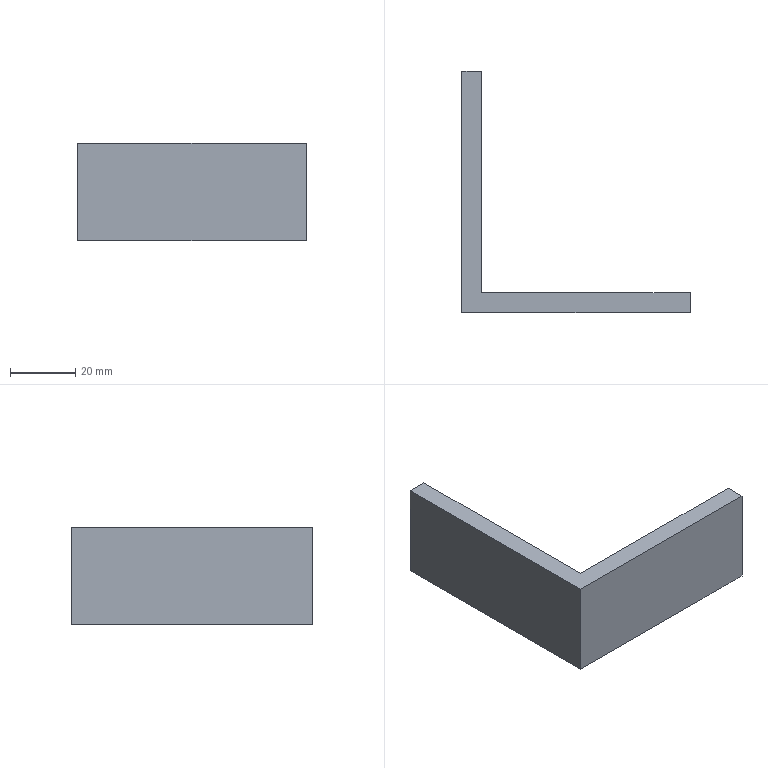Part | SolidWorks | features Extrusion 1 | 1 solid | 8 faces | box 70 x 74 x 30 mm | volume 24840 mm3 | plane 8
STEP:
#1=CARTESIAN_POINT('',(0.,74.,15.));
#2=VERTEX_POINT('',#1);
#3=CARTESIAN_POINT('',(0.,0.,15.));
#4=VERTEX_POINT('',#3);
#5=CARTESIAN_POINT('',(0.,74.,15.));
#6=DIRECTION('',(0.,-1.,0.));
#7=VECTOR('',#6,1000.);
#8=LINE('',#5,#7);
#9=EDGE_CURVE('',#2,#4,#8,.T.);
#10=ORIENTED_EDGE('',*,*,#9,.F.);
#11=CARTESIAN_POINT('',(0.,74.,-15.));
#12=VERTEX_POINT('',#11);
#13=CARTESIAN_POINT('',(0.,74.,-15.));
#14=DIRECTION('',(0.,0.,1.));
#15=VECTOR('',#14,1000.);
#16=LINE('',#13,#15);
#17=EDGE_CURVE('',#12,#2,#16,.T.);
#18=ORIENTED_EDGE('',*,*,#17,.F.);
#19=CARTESIAN_POINT('',(0.,0.,-15.));
#20=VERTEX_POINT('',#19);
#21=CARTESIAN_POINT('',(0.,74.,-15.));
#22=DIRECTION('',(0.,-1.,0.));
#23=VECTOR('',#22,1000.);
#24=LINE('',#21,#23);
#25=EDGE_CURVE('',#12,#20,#24,.T.);
#26=ORIENTED_EDGE('',*,*,#25,.T.);
#27=CARTESIAN_POINT('',(0.,0.,-15.));
#28=DIRECTION('',(0.,0.,1.));
#29=VECTOR('',#28,1000.);
#30=LINE('',#27,#29);
#31=EDGE_CURVE('',#20,#4,#30,.T.);
#32=ORIENTED_EDGE('',*,*,#31,.T.);
#33=EDGE_LOOP('',(#10,#18,#26,#32));
#34=FACE_OUTER_BOUND('',#33,.T.);
#35=CARTESIAN_POINT('',(0.,74.,-15.));
#36=DIRECTION('',(-1.,0.,0.));
#37=DIRECTION('',(0.,0.,1.));
#38=AXIS2_PLACEMENT_3D('',#35,#36,#37);
#39=PLANE('',#38);
#40=ADVANCED_FACE('',(#34),#39,.T.);
#41=CARTESIAN_POINT('',(6.,74.,15.));
#42=VERTEX_POINT('',#41);
#43=CARTESIAN_POINT('',(6.,74.,15.));
#44=DIRECTION('',(-1.,0.,0.));
#45=VECTOR('',#44,1000.);
#46=LINE('',#43,#45);
#47=EDGE_CURVE('',#42,#2,#46,.T.);
#48=ORIENTED_EDGE('',*,*,#47,.F.);
#49=CARTESIAN_POINT('',(6.,74.,-15.));
#50=VERTEX_POINT('',#49);
#51=CARTESIAN_POINT('',(6.,74.,-15.));
#52=DIRECTION('',(0.,0.,1.));
#53=VECTOR('',#52,1000.);
#54=LINE('',#51,#53);
#55=EDGE_CURVE('',#50,#42,#54,.T.);
#56=ORIENTED_EDGE('',*,*,#55,.F.);
#57=CARTESIAN_POINT('',(6.,74.,-15.));
#58=DIRECTION('',(-1.,0.,0.));
#59=VECTOR('',#58,1000.);
#60=LINE('',#57,#59);
#61=EDGE_CURVE('',#50,#12,#60,.T.);
#62=ORIENTED_EDGE('',*,*,#61,.T.);
#63=ORIENTED_EDGE('',*,*,#17,.T.);
#64=EDGE_LOOP('',(#48,#56,#62,#63));
#65=FACE_OUTER_BOUND('',#64,.T.);
#66=CARTESIAN_POINT('',(6.,74.,-15.));
#67=DIRECTION('',(0.,1.,0.));
#68=DIRECTION('',(0.,0.,1.));
#69=AXIS2_PLACEMENT_3D('',#66,#67,#68);
#70=PLANE('',#69);
#71=ADVANCED_FACE('',(#65),#70,.T.);
#72=CARTESIAN_POINT('',(6.,6.,15.));
#73=VERTEX_POINT('',#72);
#74=CARTESIAN_POINT('',(6.,6.,15.));
#75=DIRECTION('',(0.,1.,0.));
#76=VECTOR('',#75,1000.);
#77=LINE('',#74,#76);
#78=EDGE_CURVE('',#73,#42,#77,.T.);
#79=ORIENTED_EDGE('',*,*,#78,.F.);
#80=CARTESIAN_POINT('',(6.,6.,-15.));
#81=VERTEX_POINT('',#80);
#82=CARTESIAN_POINT('',(6.,6.,-15.));
#83=DIRECTION('',(0.,0.,1.));
#84=VECTOR('',#83,1000.);
#85=LINE('',#82,#84);
#86=EDGE_CURVE('',#81,#73,#85,.T.);
#87=ORIENTED_EDGE('',*,*,#86,.F.);
#88=CARTESIAN_POINT('',(6.,6.,-15.));
#89=DIRECTION('',(0.,1.,0.));
#90=VECTOR('',#89,1000.);
#91=LINE('',#88,#90);
#92=EDGE_CURVE('',#81,#50,#91,.T.);
#93=ORIENTED_EDGE('',*,*,#92,.T.);
#94=ORIENTED_EDGE('',*,*,#55,.T.);
#95=EDGE_LOOP('',(#79,#87,#93,#94));
#96=FACE_OUTER_BOUND('',#95,.T.);
#97=CARTESIAN_POINT('',(6.,6.,-15.));
#98=DIRECTION('',(1.,0.,0.));
#99=DIRECTION('',(0.,0.,-1.));
#100=AXIS2_PLACEMENT_3D('',#97,#98,#99);
#101=PLANE('',#100);
#102=ADVANCED_FACE('',(#96),#101,.T.);
#103=CARTESIAN_POINT('',(70.,6.,15.));
#104=VERTEX_POINT('',#103);
#105=CARTESIAN_POINT('',(70.,6.,15.));
#106=DIRECTION('',(-1.,0.,0.));
#107=VECTOR('',#106,1000.);
#108=LINE('',#105,#107);
#109=EDGE_CURVE('',#104,#73,#108,.T.);
#110=ORIENTED_EDGE('',*,*,#109,.F.);
#111=CARTESIAN_POINT('',(70.,6.,-15.));
#112=VERTEX_POINT('',#111);
#113=CARTESIAN_POINT('',(70.,6.,-15.));
#114=DIRECTION('',(0.,0.,1.));
#115=VECTOR('',#114,1000.);
#116=LINE('',#113,#115);
#117=EDGE_CURVE('',#112,#104,#116,.T.);
#118=ORIENTED_EDGE('',*,*,#117,.F.);
#119=CARTESIAN_POINT('',(70.,6.,-15.));
#120=DIRECTION('',(-1.,0.,0.));
#121=VECTOR('',#120,1000.);
#122=LINE('',#119,#121);
#123=EDGE_CURVE('',#112,#81,#122,.T.);
#124=ORIENTED_EDGE('',*,*,#123,.T.);
#125=ORIENTED_EDGE('',*,*,#86,.T.);
#126=EDGE_LOOP('',(#110,#118,#124,#125));
#127=FACE_OUTER_BOUND('',#126,.T.);
#128=CARTESIAN_POINT('',(70.,6.,-15.));
#129=DIRECTION('',(0.,1.,0.));
#130=DIRECTION('',(0.,0.,1.));
#131=AXIS2_PLACEMENT_3D('',#128,#129,#130);
#132=PLANE('',#131);
#133=ADVANCED_FACE('',(#127),#132,.T.);
#134=CARTESIAN_POINT('',(70.,0.,15.));
#135=VERTEX_POINT('',#134);
#136=CARTESIAN_POINT('',(70.,0.,15.));
#137=DIRECTION('',(0.,1.,0.));
#138=VECTOR('',#137,1000.);
#139=LINE('',#136,#138);
#140=EDGE_CURVE('',#135,#104,#139,.T.);
#141=ORIENTED_EDGE('',*,*,#140,.F.);
#142=CARTESIAN_POINT('',(70.,0.,-15.));
#143=VERTEX_POINT('',#142);
#144=CARTESIAN_POINT('',(70.,0.,-15.));
#145=DIRECTION('',(0.,0.,1.));
#146=VECTOR('',#145,1000.);
#147=LINE('',#144,#146);
#148=EDGE_CURVE('',#143,#135,#147,.T.);
#149=ORIENTED_EDGE('',*,*,#148,.F.);
#150=CARTESIAN_POINT('',(70.,0.,-15.));
#151=DIRECTION('',(0.,1.,0.));
#152=VECTOR('',#151,1000.);
#153=LINE('',#150,#152);
#154=EDGE_CURVE('',#143,#112,#153,.T.);
#155=ORIENTED_EDGE('',*,*,#154,.T.);
#156=ORIENTED_EDGE('',*,*,#117,.T.);
#157=EDGE_LOOP('',(#141,#149,#155,#156));
#158=FACE_OUTER_BOUND('',#157,.T.);
#159=CARTESIAN_POINT('',(70.,0.,-15.));
#160=DIRECTION('',(1.,0.,0.));
#161=DIRECTION('',(0.,0.,-1.));
#162=AXIS2_PLACEMENT_3D('',#159,#160,#161);
#163=PLANE('',#162);
#164=ADVANCED_FACE('',(#158),#163,.T.);
#165=CARTESIAN_POINT('',(0.,0.,15.));
#166=DIRECTION('',(1.,0.,0.));
#167=VECTOR('',#166,1000.);
#168=LINE('',#165,#167);
#169=EDGE_CURVE('',#4,#135,#168,.T.);
#170=ORIENTED_EDGE('',*,*,#169,.F.);
#171=ORIENTED_EDGE('',*,*,#31,.F.);
#172=CARTESIAN_POINT('',(0.,0.,-15.));
#173=DIRECTION('',(1.,0.,0.));
#174=VECTOR('',#173,1000.);
#175=LINE('',#172,#174);
#176=EDGE_CURVE('',#20,#143,#175,.T.);
#177=ORIENTED_EDGE('',*,*,#176,.T.);
#178=ORIENTED_EDGE('',*,*,#148,.T.);
#179=EDGE_LOOP('',(#170,#171,#177,#178));
#180=FACE_OUTER_BOUND('',#179,.T.);
#181=CARTESIAN_POINT('',(0.,0.,-15.));
#182=DIRECTION('',(0.,-1.,0.));
#183=DIRECTION('',(0.,0.,-1.));
#184=AXIS2_PLACEMENT_3D('',#181,#182,#183);
#185=PLANE('',#184);
#186=ADVANCED_FACE('',(#180),#185,.T.);
#187=ORIENTED_EDGE('',*,*,#25,.F.);
#188=ORIENTED_EDGE('',*,*,#61,.F.);
#189=ORIENTED_EDGE('',*,*,#92,.F.);
#190=ORIENTED_EDGE('',*,*,#123,.F.);
#191=ORIENTED_EDGE('',*,*,#154,.F.);
#192=ORIENTED_EDGE('',*,*,#176,.F.);
#193=EDGE_LOOP('',(#187,#188,#189,#190,#191,#192));
#194=FACE_OUTER_BOUND('',#193,.T.);
#195=CARTESIAN_POINT('',(0.,0.,-15.));
#196=DIRECTION('',(0.,0.,1.));
#197=DIRECTION('',(1.,0.,0.));
#198=AXIS2_PLACEMENT_3D('',#195,#196,#197);
#199=PLANE('',#198);
#200=ADVANCED_FACE('',(#194),#199,.F.);
#201=ORIENTED_EDGE('',*,*,#9,.T.);
#202=ORIENTED_EDGE('',*,*,#169,.T.);
#203=ORIENTED_EDGE('',*,*,#140,.T.);
#204=ORIENTED_EDGE('',*,*,#109,.T.);
#205=ORIENTED_EDGE('',*,*,#78,.T.);
#206=ORIENTED_EDGE('',*,*,#47,.T.);
#207=EDGE_LOOP('',(#201,#202,#203,#204,#205,#206));
#208=FACE_OUTER_BOUND('',#207,.T.);
#209=CARTESIAN_POINT('',(0.,0.,15.));
#210=DIRECTION('',(0.,0.,1.));
#211=DIRECTION('',(1.,0.,0.));
#212=AXIS2_PLACEMENT_3D('',#209,#210,#211);
#213=PLANE('',#212);
#214=ADVANCED_FACE('',(#208),#213,.T.);
#215=CLOSED_SHELL('',(#40,#71,#102,#133,#164,#186,#200,#214));
#216=MANIFOLD_SOLID_BREP('',#215);
#217=CARTESIAN_POINT('',(0.,0.,0.));
#218=DIRECTION('',(0.,0.,1.));
#219=DIRECTION('',(1.,0.,0.));
#220=AXIS2_PLACEMENT_3D('',#217,#218,#219);
#221=(LENGTH_UNIT()NAMED_UNIT(*)SI_UNIT(.MILLI.,.METRE.));
#222=UNCERTAINTY_MEASURE_WITH_UNIT(LENGTH_MEASURE(0.00001),#221,'','');
#223=(NAMED_UNIT(*)PLANE_ANGLE_UNIT()SI_UNIT($,.RADIAN.));
#224=(NAMED_UNIT(*)SI_UNIT($,.STERADIAN.)SOLID_ANGLE_UNIT());
#225=(GEOMETRIC_REPRESENTATION_CONTEXT(3)GLOBAL_UNCERTAINTY_ASSIGNED_CONTEXT((#222))GLOBAL_UNIT_ASSIGNED_CONTEXT((#221,#223,#224))REPRESENTATION_CONTEXT('',''));
#226=ADVANCED_BREP_SHAPE_REPRESENTATION('',(#216,#220),#225);